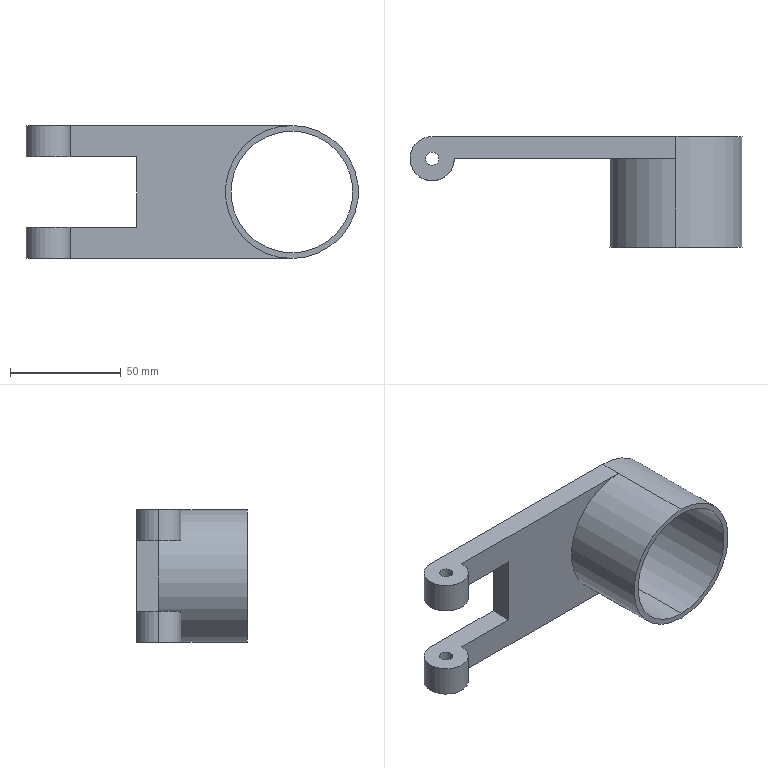Part | SolidWorks | features ICE 4, Extrusion 1 | 1 solid | 20 faces | box 150 x 50 x 60 mm | volume 67449 mm3 | cylinder 12 | plane 8 | commonest cylinder face diameters 6 x4 20 x4 55 x2 60 x2
STEP:
#1=CARTESIAN_POINT('',(110.,-40.,2.5));
#2=VERTEX_POINT('',#1);
#3=CARTESIAN_POINT('',(110.,-40.,57.5));
#4=VERTEX_POINT('',#3);
#5=CARTESIAN_POINT('',(110.,-40.,30.));
#6=DIRECTION('',(0.,1.,0.));
#7=DIRECTION('',(0.,0.,1.));
#8=AXIS2_PLACEMENT_3D('',#5,#6,#7);
#9=CIRCLE('',#8,27.5);
#10=EDGE_CURVE('',#2,#4,#9,.T.);
#11=ORIENTED_EDGE('',*,*,#10,.F.);
#12=CARTESIAN_POINT('',(110.,10.,2.5));
#13=VERTEX_POINT('',#12);
#14=CARTESIAN_POINT('',(110.,-40.,2.5));
#15=DIRECTION('',(0.,1.,0.));
#16=VECTOR('',#15,1000.);
#17=LINE('',#14,#16);
#18=EDGE_CURVE('',#2,#13,#17,.T.);
#19=ORIENTED_EDGE('',*,*,#18,.T.);
#20=CARTESIAN_POINT('',(110.,10.,57.5));
#21=VERTEX_POINT('',#20);
#22=CARTESIAN_POINT('',(110.,10.,30.));
#23=DIRECTION('',(0.,1.,0.));
#24=DIRECTION('',(0.,0.,1.));
#25=AXIS2_PLACEMENT_3D('',#22,#23,#24);
#26=CIRCLE('',#25,27.5);
#27=EDGE_CURVE('',#13,#21,#26,.T.);
#28=ORIENTED_EDGE('',*,*,#27,.T.);
#29=CARTESIAN_POINT('',(110.,-40.,57.5));
#30=DIRECTION('',(0.,1.,0.));
#31=VECTOR('',#30,1000.);
#32=LINE('',#29,#31);
#33=EDGE_CURVE('',#4,#21,#32,.T.);
#34=ORIENTED_EDGE('',*,*,#33,.F.);
#35=EDGE_LOOP('',(#11,#19,#28,#34));
#36=FACE_OUTER_BOUND('',#35,.T.);
#37=CARTESIAN_POINT('',(110.,-40.,30.));
#38=DIRECTION('',(0.,1.,0.));
#39=DIRECTION('',(0.,0.,1.));
#40=AXIS2_PLACEMENT_3D('',#37,#38,#39);
#41=CYLINDRICAL_SURFACE('',#40,27.5);
#42=ADVANCED_FACE('',(#36),#41,.F.);
#43=CARTESIAN_POINT('',(110.,-40.,60.));
#44=VERTEX_POINT('',#43);
#45=CARTESIAN_POINT('',(110.,-40.,0.));
#46=VERTEX_POINT('',#45);
#47=CARTESIAN_POINT('',(110.,-40.,30.));
#48=DIRECTION('',(0.,1.,0.));
#49=DIRECTION('',(0.,0.,1.));
#50=AXIS2_PLACEMENT_3D('',#47,#48,#49);
#51=CIRCLE('',#50,30.);
#52=EDGE_CURVE('',#44,#46,#51,.T.);
#53=ORIENTED_EDGE('',*,*,#52,.T.);
#54=CARTESIAN_POINT('',(110.,0.,0.));
#55=VERTEX_POINT('',#54);
#56=CARTESIAN_POINT('',(110.,-40.,0.));
#57=DIRECTION('',(0.,1.,0.));
#58=VECTOR('',#57,1000.);
#59=LINE('',#56,#58);
#60=EDGE_CURVE('',#46,#55,#59,.T.);
#61=ORIENTED_EDGE('',*,*,#60,.T.);
#62=CARTESIAN_POINT('',(110.,10.,0.));
#63=VERTEX_POINT('',#62);
#64=CARTESIAN_POINT('',(110.,10.,0.));
#65=DIRECTION('',(0.,-1.,0.));
#66=VECTOR('',#65,1000.);
#67=LINE('',#64,#66);
#68=EDGE_CURVE('',#63,#55,#67,.T.);
#69=ORIENTED_EDGE('',*,*,#68,.F.);
#70=CARTESIAN_POINT('',(110.,10.,60.));
#71=VERTEX_POINT('',#70);
#72=CARTESIAN_POINT('',(110.,10.,30.));
#73=DIRECTION('',(0.,1.,0.));
#74=DIRECTION('',(0.,0.,1.));
#75=AXIS2_PLACEMENT_3D('',#72,#73,#74);
#76=CIRCLE('',#75,30.);
#77=EDGE_CURVE('',#71,#63,#76,.T.);
#78=ORIENTED_EDGE('',*,*,#77,.F.);
#79=CARTESIAN_POINT('',(110.,0.,60.));
#80=VERTEX_POINT('',#79);
#81=CARTESIAN_POINT('',(110.,10.,60.));
#82=DIRECTION('',(0.,1.,0.));
#83=VECTOR('',#82,1000.);
#84=LINE('',#81,#83);
#85=EDGE_CURVE('',#80,#71,#84,.T.);
#86=ORIENTED_EDGE('',*,*,#85,.F.);
#87=CARTESIAN_POINT('',(110.,-40.,60.));
#88=DIRECTION('',(0.,1.,0.));
#89=VECTOR('',#88,1000.);
#90=LINE('',#87,#89);
#91=EDGE_CURVE('',#44,#80,#90,.T.);
#92=ORIENTED_EDGE('',*,*,#91,.F.);
#93=EDGE_LOOP('',(#53,#61,#69,#78,#86,#92));
#94=FACE_OUTER_BOUND('',#93,.T.);
#95=CARTESIAN_POINT('',(110.,-40.,30.));
#96=DIRECTION('',(0.,1.,0.));
#97=DIRECTION('',(0.,0.,1.));
#98=AXIS2_PLACEMENT_3D('',#95,#96,#97);
#99=CYLINDRICAL_SURFACE('',#98,30.);
#100=ADVANCED_FACE('',(#94),#99,.T.);
#101=CARTESIAN_POINT('',(3.,0.,14.));
#102=VERTEX_POINT('',#101);
#103=CARTESIAN_POINT('',(-3.,0.,14.));
#104=VERTEX_POINT('',#103);
#105=CARTESIAN_POINT('',(0.,0.,14.));
#106=DIRECTION('',(0.,0.,-1.));
#107=DIRECTION('',(-1.,0.,0.));
#108=AXIS2_PLACEMENT_3D('',#105,#106,#107);
#109=CIRCLE('',#108,3.);
#110=EDGE_CURVE('',#102,#104,#109,.T.);
#111=ORIENTED_EDGE('',*,*,#110,.F.);
#112=CARTESIAN_POINT('',(3.,0.,0.));
#113=VERTEX_POINT('',#112);
#114=CARTESIAN_POINT('',(3.,0.,60.));
#115=DIRECTION('',(0.,0.,-1.));
#116=VECTOR('',#115,1000.);
#117=LINE('',#114,#116);
#118=EDGE_CURVE('',#102,#113,#117,.T.);
#119=ORIENTED_EDGE('',*,*,#118,.T.);
#120=CARTESIAN_POINT('',(-3.,0.,0.));
#121=VERTEX_POINT('',#120);
#122=CARTESIAN_POINT('',(0.,0.,0.));
#123=DIRECTION('',(0.,0.,1.));
#124=DIRECTION('',(1.,0.,0.));
#125=AXIS2_PLACEMENT_3D('',#122,#123,#124);
#126=CIRCLE('',#125,3.);
#127=EDGE_CURVE('',#121,#113,#126,.T.);
#128=ORIENTED_EDGE('',*,*,#127,.F.);
#129=CARTESIAN_POINT('',(-3.,0.,60.));
#130=DIRECTION('',(0.,0.,-1.));
#131=VECTOR('',#130,1000.);
#132=LINE('',#129,#131);
#133=EDGE_CURVE('',#104,#121,#132,.T.);
#134=ORIENTED_EDGE('',*,*,#133,.F.);
#135=EDGE_LOOP('',(#111,#119,#128,#134));
#136=FACE_OUTER_BOUND('',#135,.T.);
#137=CARTESIAN_POINT('',(0.,0.,60.));
#138=DIRECTION('',(0.,0.,-1.));
#139=DIRECTION('',(-1.,0.,0.));
#140=AXIS2_PLACEMENT_3D('',#137,#138,#139);
#141=CYLINDRICAL_SURFACE('',#140,3.);
#142=ADVANCED_FACE('',(#136),#141,.F.);
#143=CARTESIAN_POINT('',(-10.,0.,60.));
#144=VERTEX_POINT('',#143);
#145=CARTESIAN_POINT('',(10.,0.,60.));
#146=VERTEX_POINT('',#145);
#147=CARTESIAN_POINT('',(0.,0.,60.));
#148=DIRECTION('',(0.,0.,1.));
#149=DIRECTION('',(1.,0.,0.));
#150=AXIS2_PLACEMENT_3D('',#147,#148,#149);
#151=CIRCLE('',#150,10.);
#152=EDGE_CURVE('',#144,#146,#151,.T.);
#153=ORIENTED_EDGE('',*,*,#152,.F.);
#154=CARTESIAN_POINT('',(-10.,0.,46.));
#155=VERTEX_POINT('',#154);
#156=CARTESIAN_POINT('',(-10.,0.,60.));
#157=DIRECTION('',(0.,0.,-1.));
#158=VECTOR('',#157,1000.);
#159=LINE('',#156,#158);
#160=EDGE_CURVE('',#144,#155,#159,.T.);
#161=ORIENTED_EDGE('',*,*,#160,.T.);
#162=CARTESIAN_POINT('',(10.,0.,46.));
#163=VERTEX_POINT('',#162);
#164=CARTESIAN_POINT('',(0.,0.,46.));
#165=DIRECTION('',(0.,0.,1.));
#166=DIRECTION('',(1.,0.,0.));
#167=AXIS2_PLACEMENT_3D('',#164,#165,#166);
#168=CIRCLE('',#167,10.);
#169=EDGE_CURVE('',#155,#163,#168,.T.);
#170=ORIENTED_EDGE('',*,*,#169,.T.);
#171=CARTESIAN_POINT('',(10.,0.,-110.454));
#172=DIRECTION('',(0.,0.,1.));
#173=VECTOR('',#172,1000.);
#174=LINE('',#171,#173);
#175=EDGE_CURVE('',#163,#146,#174,.T.);
#176=ORIENTED_EDGE('',*,*,#175,.T.);
#177=EDGE_LOOP('',(#153,#161,#170,#176));
#178=FACE_OUTER_BOUND('',#177,.T.);
#179=CARTESIAN_POINT('',(0.,0.,60.));
#180=DIRECTION('',(0.,0.,-1.));
#181=DIRECTION('',(-1.,0.,0.));
#182=AXIS2_PLACEMENT_3D('',#179,#180,#181);
#183=CYLINDRICAL_SURFACE('',#182,10.);
#184=ADVANCED_FACE('',(#178),#183,.T.);
#185=CARTESIAN_POINT('',(-3.,0.,60.));
#186=VERTEX_POINT('',#185);
#187=CARTESIAN_POINT('',(3.,0.,60.));
#188=VERTEX_POINT('',#187);
#189=CARTESIAN_POINT('',(0.,0.,60.));
#190=DIRECTION('',(0.,0.,1.));
#191=DIRECTION('',(1.,0.,0.));
#192=AXIS2_PLACEMENT_3D('',#189,#190,#191);
#193=CIRCLE('',#192,3.);
#194=EDGE_CURVE('',#186,#188,#193,.T.);
#195=ORIENTED_EDGE('',*,*,#194,.T.);
#196=CARTESIAN_POINT('',(3.,0.,46.));
#197=VERTEX_POINT('',#196);
#198=CARTESIAN_POINT('',(3.,0.,60.));
#199=DIRECTION('',(0.,0.,-1.));
#200=VECTOR('',#199,1000.);
#201=LINE('',#198,#200);
#202=EDGE_CURVE('',#188,#197,#201,.T.);
#203=ORIENTED_EDGE('',*,*,#202,.T.);
#204=CARTESIAN_POINT('',(-3.,0.,46.));
#205=VERTEX_POINT('',#204);
#206=CARTESIAN_POINT('',(0.,0.,46.));
#207=DIRECTION('',(0.,0.,1.));
#208=DIRECTION('',(1.,0.,0.));
#209=AXIS2_PLACEMENT_3D('',#206,#207,#208);
#210=CIRCLE('',#209,3.);
#211=EDGE_CURVE('',#205,#197,#210,.T.);
#212=ORIENTED_EDGE('',*,*,#211,.F.);
#213=CARTESIAN_POINT('',(-3.,0.,60.));
#214=DIRECTION('',(0.,0.,-1.));
#215=VECTOR('',#214,1000.);
#216=LINE('',#213,#215);
#217=EDGE_CURVE('',#186,#205,#216,.T.);
#218=ORIENTED_EDGE('',*,*,#217,.F.);
#219=EDGE_LOOP('',(#195,#203,#212,#218));
#220=FACE_OUTER_BOUND('',#219,.T.);
#221=CARTESIAN_POINT('',(0.,0.,60.));
#222=DIRECTION('',(0.,0.,-1.));
#223=DIRECTION('',(-1.,0.,0.));
#224=AXIS2_PLACEMENT_3D('',#221,#222,#223);
#225=CYLINDRICAL_SURFACE('',#224,3.);
#226=ADVANCED_FACE('',(#220),#225,.F.);
#227=CARTESIAN_POINT('',(10.,0.,14.));
#228=VERTEX_POINT('',#227);
#229=CARTESIAN_POINT('',(-10.,0.,14.));
#230=VERTEX_POINT('',#229);
#231=CARTESIAN_POINT('',(0.,0.,14.));
#232=DIRECTION('',(0.,0.,-1.));
#233=DIRECTION('',(-1.,0.,0.));
#234=AXIS2_PLACEMENT_3D('',#231,#232,#233);
#235=CIRCLE('',#234,10.);
#236=EDGE_CURVE('',#228,#230,#235,.T.);
#237=ORIENTED_EDGE('',*,*,#236,.T.);
#238=CARTESIAN_POINT('',(-10.,0.,0.));
#239=VERTEX_POINT('',#238);
#240=CARTESIAN_POINT('',(-10.,0.,60.));
#241=DIRECTION('',(0.,0.,-1.));
#242=VECTOR('',#241,1000.);
#243=LINE('',#240,#242);
#244=EDGE_CURVE('',#230,#239,#243,.T.);
#245=ORIENTED_EDGE('',*,*,#244,.T.);
#246=CARTESIAN_POINT('',(10.,0.,0.));
#247=VERTEX_POINT('',#246);
#248=CARTESIAN_POINT('',(0.,0.,0.));
#249=DIRECTION('',(0.,0.,1.));
#250=DIRECTION('',(1.,0.,0.));
#251=AXIS2_PLACEMENT_3D('',#248,#249,#250);
#252=CIRCLE('',#251,10.);
#253=EDGE_CURVE('',#239,#247,#252,.T.);
#254=ORIENTED_EDGE('',*,*,#253,.T.);
#255=CARTESIAN_POINT('',(10.,0.,-110.454));
#256=DIRECTION('',(0.,0.,1.));
#257=VECTOR('',#256,1000.);
#258=LINE('',#255,#257);
#259=EDGE_CURVE('',#247,#228,#258,.T.);
#260=ORIENTED_EDGE('',*,*,#259,.T.);
#261=EDGE_LOOP('',(#237,#245,#254,#260));
#262=FACE_OUTER_BOUND('',#261,.T.);
#263=CARTESIAN_POINT('',(0.,0.,60.));
#264=DIRECTION('',(0.,0.,-1.));
#265=DIRECTION('',(-1.,0.,0.));
#266=AXIS2_PLACEMENT_3D('',#263,#264,#265);
#267=CYLINDRICAL_SURFACE('',#266,10.);
#268=ADVANCED_FACE('',(#262),#267,.T.);
#269=ORIENTED_EDGE('',*,*,#244,.F.);
#270=CARTESIAN_POINT('',(0.,10.,14.));
#271=VERTEX_POINT('',#270);
#272=CARTESIAN_POINT('',(0.,0.,14.));
#273=DIRECTION('',(0.,0.,-1.));
#274=DIRECTION('',(-1.,0.,0.));
#275=AXIS2_PLACEMENT_3D('',#272,#273,#274);
#276=CIRCLE('',#275,10.);
#277=EDGE_CURVE('',#230,#271,#276,.T.);
#278=ORIENTED_EDGE('',*,*,#277,.T.);
#279=CARTESIAN_POINT('',(0.,10.,0.));
#280=VERTEX_POINT('',#279);
#281=CARTESIAN_POINT('',(0.,10.,-110.454));
#282=DIRECTION('',(0.,0.,1.));
#283=VECTOR('',#282,1000.);
#284=LINE('',#281,#283);
#285=EDGE_CURVE('',#280,#271,#284,.T.);
#286=ORIENTED_EDGE('',*,*,#285,.F.);
#287=CARTESIAN_POINT('',(0.,0.,0.));
#288=DIRECTION('',(0.,0.,1.));
#289=DIRECTION('',(1.,0.,0.));
#290=AXIS2_PLACEMENT_3D('',#287,#288,#289);
#291=CIRCLE('',#290,10.);
#292=EDGE_CURVE('',#280,#239,#291,.T.);
#293=ORIENTED_EDGE('',*,*,#292,.T.);
#294=EDGE_LOOP('',(#269,#278,#286,#293));
#295=FACE_OUTER_BOUND('',#294,.T.);
#296=CARTESIAN_POINT('',(0.,0.,60.));
#297=DIRECTION('',(0.,0.,-1.));
#298=DIRECTION('',(-1.,0.,0.));
#299=AXIS2_PLACEMENT_3D('',#296,#297,#298);
#300=CYLINDRICAL_SURFACE('',#299,10.);
#301=ADVANCED_FACE('',(#295),#300,.T.);
#302=ORIENTED_EDGE('',*,*,#202,.F.);
#303=CARTESIAN_POINT('',(0.,0.,60.));
#304=DIRECTION('',(0.,0.,1.));
#305=DIRECTION('',(1.,0.,0.));
#306=AXIS2_PLACEMENT_3D('',#303,#304,#305);
#307=CIRCLE('',#306,3.);
#308=EDGE_CURVE('',#188,#186,#307,.T.);
#309=ORIENTED_EDGE('',*,*,#308,.T.);
#310=ORIENTED_EDGE('',*,*,#217,.T.);
#311=CARTESIAN_POINT('',(0.,0.,46.));
#312=DIRECTION('',(0.,0.,1.));
#313=DIRECTION('',(1.,0.,0.));
#314=AXIS2_PLACEMENT_3D('',#311,#312,#313);
#315=CIRCLE('',#314,3.);
#316=EDGE_CURVE('',#197,#205,#315,.T.);
#317=ORIENTED_EDGE('',*,*,#316,.F.);
#318=EDGE_LOOP('',(#302,#309,#310,#317));
#319=FACE_OUTER_BOUND('',#318,.T.);
#320=CARTESIAN_POINT('',(0.,0.,60.));
#321=DIRECTION('',(0.,0.,-1.));
#322=DIRECTION('',(-1.,0.,0.));
#323=AXIS2_PLACEMENT_3D('',#320,#321,#322);
#324=CYLINDRICAL_SURFACE('',#323,3.);
#325=ADVANCED_FACE('',(#319),#324,.F.);
#326=CARTESIAN_POINT('',(0.,10.,60.));
#327=VERTEX_POINT('',#326);
#328=CARTESIAN_POINT('',(0.,0.,60.));
#329=DIRECTION('',(0.,0.,1.));
#330=DIRECTION('',(1.,0.,0.));
#331=AXIS2_PLACEMENT_3D('',#328,#329,#330);
#332=CIRCLE('',#331,10.);
#333=EDGE_CURVE('',#327,#144,#332,.T.);
#334=ORIENTED_EDGE('',*,*,#333,.T.);
#335=ORIENTED_EDGE('',*,*,#152,.T.);
#336=CARTESIAN_POINT('',(10.,0.,60.));
#337=DIRECTION('',(1.,0.,0.));
#338=VECTOR('',#337,1000.);
#339=LINE('',#336,#338);
#340=EDGE_CURVE('',#146,#80,#339,.T.);
#341=ORIENTED_EDGE('',*,*,#340,.T.);
#342=ORIENTED_EDGE('',*,*,#85,.T.);
#343=CARTESIAN_POINT('',(0.,10.,60.));
#344=DIRECTION('',(-1.,0.,0.));
#345=VECTOR('',#344,1000.);
#346=LINE('',#343,#345);
#347=EDGE_CURVE('',#71,#327,#346,.T.);
#348=ORIENTED_EDGE('',*,*,#347,.T.);
#349=EDGE_LOOP('',(#334,#335,#341,#342,#348));
#350=FACE_OUTER_BOUND('',#349,.T.);
#351=ORIENTED_EDGE('',*,*,#194,.F.);
#352=ORIENTED_EDGE('',*,*,#308,.F.);
#353=EDGE_LOOP('',(#351,#352));
#354=FACE_BOUND('',#353,.T.);
#355=CARTESIAN_POINT('',(0.,0.,60.));
#356=DIRECTION('',(0.,0.,1.));
#357=DIRECTION('',(1.,0.,0.));
#358=AXIS2_PLACEMENT_3D('',#355,#356,#357);
#359=PLANE('',#358);
#360=ADVANCED_FACE('',(#350,#354),#359,.T.);
#361=ORIENTED_EDGE('',*,*,#292,.F.);
#362=CARTESIAN_POINT('',(0.,10.,0.));
#363=DIRECTION('',(1.,0.,0.));
#364=VECTOR('',#363,1000.);
#365=LINE('',#362,#364);
#366=EDGE_CURVE('',#280,#63,#365,.T.);
#367=ORIENTED_EDGE('',*,*,#366,.T.);
#368=ORIENTED_EDGE('',*,*,#68,.T.);
#369=CARTESIAN_POINT('',(10.,0.,0.));
#370=DIRECTION('',(-1.,0.,0.));
#371=VECTOR('',#370,1000.);
#372=LINE('',#369,#371);
#373=EDGE_CURVE('',#55,#247,#372,.T.);
#374=ORIENTED_EDGE('',*,*,#373,.T.);
#375=ORIENTED_EDGE('',*,*,#253,.F.);
#376=EDGE_LOOP('',(#361,#367,#368,#374,#375));
#377=FACE_OUTER_BOUND('',#376,.T.);
#378=ORIENTED_EDGE('',*,*,#127,.T.);
#379=CARTESIAN_POINT('',(0.,0.,0.));
#380=DIRECTION('',(0.,0.,1.));
#381=DIRECTION('',(1.,0.,0.));
#382=AXIS2_PLACEMENT_3D('',#379,#380,#381);
#383=CIRCLE('',#382,3.);
#384=EDGE_CURVE('',#113,#121,#383,.T.);
#385=ORIENTED_EDGE('',*,*,#384,.T.);
#386=EDGE_LOOP('',(#378,#385));
#387=FACE_BOUND('',#386,.T.);
#388=CARTESIAN_POINT('',(0.,0.,0.));
#389=DIRECTION('',(0.,0.,1.));
#390=DIRECTION('',(1.,0.,0.));
#391=AXIS2_PLACEMENT_3D('',#388,#389,#390);
#392=PLANE('',#391);
#393=ADVANCED_FACE('',(#377,#387),#392,.F.);
#394=ORIENTED_EDGE('',*,*,#160,.F.);
#395=ORIENTED_EDGE('',*,*,#333,.F.);
#396=CARTESIAN_POINT('',(0.,10.,46.));
#397=VERTEX_POINT('',#396);
#398=CARTESIAN_POINT('',(0.,10.,-110.454));
#399=DIRECTION('',(0.,0.,1.));
#400=VECTOR('',#399,1000.);
#401=LINE('',#398,#400);
#402=EDGE_CURVE('',#397,#327,#401,.T.);
#403=ORIENTED_EDGE('',*,*,#402,.F.);
#404=CARTESIAN_POINT('',(0.,0.,46.));
#405=DIRECTION('',(0.,0.,1.));
#406=DIRECTION('',(1.,0.,0.));
#407=AXIS2_PLACEMENT_3D('',#404,#405,#406);
#408=CIRCLE('',#407,10.);
#409=EDGE_CURVE('',#397,#155,#408,.T.);
#410=ORIENTED_EDGE('',*,*,#409,.T.);
#411=EDGE_LOOP('',(#394,#395,#403,#410));
#412=FACE_OUTER_BOUND('',#411,.T.);
#413=CARTESIAN_POINT('',(0.,0.,60.));
#414=DIRECTION('',(0.,0.,-1.));
#415=DIRECTION('',(-1.,0.,0.));
#416=AXIS2_PLACEMENT_3D('',#413,#414,#415);
#417=CYLINDRICAL_SURFACE('',#416,10.);
#418=ADVANCED_FACE('',(#412),#417,.T.);
#419=ORIENTED_EDGE('',*,*,#118,.F.);
#420=CARTESIAN_POINT('',(0.,0.,14.));
#421=DIRECTION('',(0.,0.,-1.));
#422=DIRECTION('',(-1.,0.,0.));
#423=AXIS2_PLACEMENT_3D('',#420,#421,#422);
#424=CIRCLE('',#423,3.);
#425=EDGE_CURVE('',#104,#102,#424,.T.);
#426=ORIENTED_EDGE('',*,*,#425,.F.);
#427=ORIENTED_EDGE('',*,*,#133,.T.);
#428=ORIENTED_EDGE('',*,*,#384,.F.);
#429=EDGE_LOOP('',(#419,#426,#427,#428));
#430=FACE_OUTER_BOUND('',#429,.T.);
#431=CARTESIAN_POINT('',(0.,0.,60.));
#432=DIRECTION('',(0.,0.,-1.));
#433=DIRECTION('',(-1.,0.,0.));
#434=AXIS2_PLACEMENT_3D('',#431,#432,#433);
#435=CYLINDRICAL_SURFACE('',#434,3.);
#436=ADVANCED_FACE('',(#430),#435,.F.);
#437=CARTESIAN_POINT('',(110.,10.,30.));
#438=DIRECTION('',(0.,1.,0.));
#439=DIRECTION('',(0.,0.,1.));
#440=AXIS2_PLACEMENT_3D('',#437,#438,#439);
#441=CIRCLE('',#440,27.5);
#442=EDGE_CURVE('',#21,#13,#441,.T.);
#443=ORIENTED_EDGE('',*,*,#442,.F.);
#444=ORIENTED_EDGE('',*,*,#27,.F.);
#445=EDGE_LOOP('',(#443,#444));
#446=FACE_BOUND('',#445,.T.);
#447=ORIENTED_EDGE('',*,*,#347,.F.);
#448=ORIENTED_EDGE('',*,*,#77,.T.);
#449=ORIENTED_EDGE('',*,*,#366,.F.);
#450=ORIENTED_EDGE('',*,*,#285,.T.);
#451=CARTESIAN_POINT('',(40.,10.,14.));
#452=VERTEX_POINT('',#451);
#453=CARTESIAN_POINT('',(0.,10.,14.));
#454=DIRECTION('',(-1.,0.,0.));
#455=VECTOR('',#454,1000.);
#456=LINE('',#453,#455);
#457=EDGE_CURVE('',#452,#271,#456,.T.);
#458=ORIENTED_EDGE('',*,*,#457,.F.);
#459=CARTESIAN_POINT('',(40.,10.,46.));
#460=VERTEX_POINT('',#459);
#461=CARTESIAN_POINT('',(40.,10.,-110.454));
#462=DIRECTION('',(0.,0.,-1.));
#463=VECTOR('',#462,1000.);
#464=LINE('',#461,#463);
#465=EDGE_CURVE('',#460,#452,#464,.T.);
#466=ORIENTED_EDGE('',*,*,#465,.F.);
#467=CARTESIAN_POINT('',(0.,10.,46.));
#468=DIRECTION('',(1.,0.,0.));
#469=VECTOR('',#468,1000.);
#470=LINE('',#467,#469);
#471=EDGE_CURVE('',#397,#460,#470,.T.);
#472=ORIENTED_EDGE('',*,*,#471,.F.);
#473=ORIENTED_EDGE('',*,*,#402,.T.);
#474=EDGE_LOOP('',(#447,#448,#449,#450,#458,#466,#472,#473));
#475=FACE_OUTER_BOUND('',#474,.T.);
#476=CARTESIAN_POINT('',(0.,10.,-110.454));
#477=DIRECTION('',(0.,1.,0.));
#478=DIRECTION('',(0.,0.,1.));
#479=AXIS2_PLACEMENT_3D('',#476,#477,#478);
#480=PLANE('',#479);
#481=ADVANCED_FACE('',(#446,#475),#480,.T.);
#482=CARTESIAN_POINT('',(110.,0.,30.));
#483=DIRECTION('',(0.,-1.,0.));
#484=DIRECTION('',(0.,0.,-1.));
#485=AXIS2_PLACEMENT_3D('',#482,#483,#484);
#486=CIRCLE('',#485,30.);
#487=EDGE_CURVE('',#80,#55,#486,.T.);
#488=ORIENTED_EDGE('',*,*,#487,.F.);
#489=ORIENTED_EDGE('',*,*,#340,.F.);
#490=ORIENTED_EDGE('',*,*,#175,.F.);
#491=CARTESIAN_POINT('',(40.,0.,46.));
#492=VERTEX_POINT('',#491);
#493=CARTESIAN_POINT('',(10.,0.,46.));
#494=DIRECTION('',(-1.,0.,0.));
#495=VECTOR('',#494,1000.);
#496=LINE('',#493,#495);
#497=EDGE_CURVE('',#492,#163,#496,.T.);
#498=ORIENTED_EDGE('',*,*,#497,.F.);
#499=CARTESIAN_POINT('',(40.,0.,14.));
#500=VERTEX_POINT('',#499);
#501=CARTESIAN_POINT('',(40.,0.,-110.454));
#502=DIRECTION('',(0.,0.,1.));
#503=VECTOR('',#502,1000.);
#504=LINE('',#501,#503);
#505=EDGE_CURVE('',#500,#492,#504,.T.);
#506=ORIENTED_EDGE('',*,*,#505,.F.);
#507=CARTESIAN_POINT('',(10.,0.,14.));
#508=DIRECTION('',(1.,0.,0.));
#509=VECTOR('',#508,1000.);
#510=LINE('',#507,#509);
#511=EDGE_CURVE('',#228,#500,#510,.T.);
#512=ORIENTED_EDGE('',*,*,#511,.F.);
#513=ORIENTED_EDGE('',*,*,#259,.F.);
#514=ORIENTED_EDGE('',*,*,#373,.F.);
#515=EDGE_LOOP('',(#488,#489,#490,#498,#506,#512,#513,#514));
#516=FACE_OUTER_BOUND('',#515,.T.);
#517=CARTESIAN_POINT('',(10.,0.,-110.454));
#518=DIRECTION('',(0.,-1.,0.));
#519=DIRECTION('',(0.,0.,-1.));
#520=AXIS2_PLACEMENT_3D('',#517,#518,#519);
#521=PLANE('',#520);
#522=ADVANCED_FACE('',(#516),#521,.T.);
#523=ORIENTED_EDGE('',*,*,#211,.T.);
#524=ORIENTED_EDGE('',*,*,#316,.T.);
#525=EDGE_LOOP('',(#523,#524));
#526=FACE_BOUND('',#525,.T.);
#527=ORIENTED_EDGE('',*,*,#471,.T.);
#528=CARTESIAN_POINT('',(40.,-10.,46.));
#529=DIRECTION('',(0.,1.,0.));
#530=VECTOR('',#529,1000.);
#531=LINE('',#528,#530);
#532=EDGE_CURVE('',#492,#460,#531,.T.);
#533=ORIENTED_EDGE('',*,*,#532,.F.);
#534=ORIENTED_EDGE('',*,*,#497,.T.);
#535=ORIENTED_EDGE('',*,*,#169,.F.);
#536=ORIENTED_EDGE('',*,*,#409,.F.);
#537=EDGE_LOOP('',(#527,#533,#534,#535,#536));
#538=FACE_OUTER_BOUND('',#537,.T.);
#539=CARTESIAN_POINT('',(-57.331,-10.,46.));
#540=DIRECTION('',(0.,0.,1.));
#541=DIRECTION('',(1.,0.,0.));
#542=AXIS2_PLACEMENT_3D('',#539,#540,#541);
#543=PLANE('',#542);
#544=ADVANCED_FACE('',(#526,#538),#543,.F.);
#545=ORIENTED_EDGE('',*,*,#425,.T.);
#546=ORIENTED_EDGE('',*,*,#110,.T.);
#547=EDGE_LOOP('',(#545,#546));
#548=FACE_BOUND('',#547,.T.);
#549=ORIENTED_EDGE('',*,*,#457,.T.);
#550=ORIENTED_EDGE('',*,*,#277,.F.);
#551=ORIENTED_EDGE('',*,*,#236,.F.);
#552=ORIENTED_EDGE('',*,*,#511,.T.);
#553=CARTESIAN_POINT('',(40.,-10.,14.));
#554=DIRECTION('',(0.,1.,0.));
#555=VECTOR('',#554,1000.);
#556=LINE('',#553,#555);
#557=EDGE_CURVE('',#500,#452,#556,.T.);
#558=ORIENTED_EDGE('',*,*,#557,.T.);
#559=EDGE_LOOP('',(#549,#550,#551,#552,#558));
#560=FACE_OUTER_BOUND('',#559,.T.);
#561=CARTESIAN_POINT('',(-57.331,-10.,14.));
#562=DIRECTION('',(0.,0.,-1.));
#563=DIRECTION('',(-1.,0.,0.));
#564=AXIS2_PLACEMENT_3D('',#561,#562,#563);
#565=PLANE('',#564);
#566=ADVANCED_FACE('',(#548,#560),#565,.F.);
#567=ORIENTED_EDGE('',*,*,#465,.T.);
#568=ORIENTED_EDGE('',*,*,#557,.F.);
#569=ORIENTED_EDGE('',*,*,#505,.T.);
#570=ORIENTED_EDGE('',*,*,#532,.T.);
#571=EDGE_LOOP('',(#567,#568,#569,#570));
#572=FACE_OUTER_BOUND('',#571,.T.);
#573=CARTESIAN_POINT('',(40.,-10.,14.));
#574=DIRECTION('',(1.,0.,0.));
#575=DIRECTION('',(0.,0.,-1.));
#576=AXIS2_PLACEMENT_3D('',#573,#574,#575);
#577=PLANE('',#576);
#578=ADVANCED_FACE('',(#572),#577,.F.);
#579=ORIENTED_EDGE('',*,*,#60,.F.);
#580=CARTESIAN_POINT('',(110.,-40.,30.));
#581=DIRECTION('',(0.,1.,0.));
#582=DIRECTION('',(0.,0.,1.));
#583=AXIS2_PLACEMENT_3D('',#580,#581,#582);
#584=CIRCLE('',#583,30.);
#585=EDGE_CURVE('',#46,#44,#584,.T.);
#586=ORIENTED_EDGE('',*,*,#585,.T.);
#587=ORIENTED_EDGE('',*,*,#91,.T.);
#588=ORIENTED_EDGE('',*,*,#487,.T.);
#589=EDGE_LOOP('',(#579,#586,#587,#588));
#590=FACE_OUTER_BOUND('',#589,.T.);
#591=CARTESIAN_POINT('',(110.,-40.,30.));
#592=DIRECTION('',(0.,1.,0.));
#593=DIRECTION('',(0.,0.,1.));
#594=AXIS2_PLACEMENT_3D('',#591,#592,#593);
#595=CYLINDRICAL_SURFACE('',#594,30.);
#596=ADVANCED_FACE('',(#590),#595,.T.);
#597=CARTESIAN_POINT('',(110.,-40.,30.));
#598=DIRECTION('',(0.,1.,0.));
#599=DIRECTION('',(0.,0.,1.));
#600=AXIS2_PLACEMENT_3D('',#597,#598,#599);
#601=CIRCLE('',#600,27.5);
#602=EDGE_CURVE('',#4,#2,#601,.T.);
#603=ORIENTED_EDGE('',*,*,#602,.T.);
#604=ORIENTED_EDGE('',*,*,#10,.T.);
#605=EDGE_LOOP('',(#603,#604));
#606=FACE_BOUND('',#605,.T.);
#607=ORIENTED_EDGE('',*,*,#52,.F.);
#608=ORIENTED_EDGE('',*,*,#585,.F.);
#609=EDGE_LOOP('',(#607,#608));
#610=FACE_OUTER_BOUND('',#609,.T.);
#611=CARTESIAN_POINT('',(110.,-40.,30.));
#612=DIRECTION('',(0.,1.,0.));
#613=DIRECTION('',(0.,0.,1.));
#614=AXIS2_PLACEMENT_3D('',#611,#612,#613);
#615=PLANE('',#614);
#616=ADVANCED_FACE('',(#606,#610),#615,.F.);
#617=ORIENTED_EDGE('',*,*,#18,.F.);
#618=ORIENTED_EDGE('',*,*,#602,.F.);
#619=ORIENTED_EDGE('',*,*,#33,.T.);
#620=ORIENTED_EDGE('',*,*,#442,.T.);
#621=EDGE_LOOP('',(#617,#618,#619,#620));
#622=FACE_OUTER_BOUND('',#621,.T.);
#623=CARTESIAN_POINT('',(110.,-40.,30.));
#624=DIRECTION('',(0.,1.,0.));
#625=DIRECTION('',(0.,0.,1.));
#626=AXIS2_PLACEMENT_3D('',#623,#624,#625);
#627=CYLINDRICAL_SURFACE('',#626,27.5);
#628=ADVANCED_FACE('',(#622),#627,.F.);
#629=CLOSED_SHELL('',(#42,#100,#142,#184,#226,#268,#301,#325,#360,#393,#418,#436,#481,#522,#544,#566,#578,#596,#616,#628));
#630=MANIFOLD_SOLID_BREP('',#629);
#631=CARTESIAN_POINT('',(0.,0.,0.));
#632=DIRECTION('',(0.,0.,1.));
#633=DIRECTION('',(1.,0.,0.));
#634=AXIS2_PLACEMENT_3D('',#631,#632,#633);
#635=(LENGTH_UNIT()NAMED_UNIT(*)SI_UNIT(.MILLI.,.METRE.));
#636=UNCERTAINTY_MEASURE_WITH_UNIT(LENGTH_MEASURE(0.00001),#635,'','');
#637=(NAMED_UNIT(*)PLANE_ANGLE_UNIT()SI_UNIT($,.RADIAN.));
#638=(NAMED_UNIT(*)SI_UNIT($,.STERADIAN.)SOLID_ANGLE_UNIT());
#639=(GEOMETRIC_REPRESENTATION_CONTEXT(3)GLOBAL_UNCERTAINTY_ASSIGNED_CONTEXT((#636))GLOBAL_UNIT_ASSIGNED_CONTEXT((#635,#637,#638))REPRESENTATION_CONTEXT('',''));
#640=ADVANCED_BREP_SHAPE_REPRESENTATION('',(#630,#634),#639);